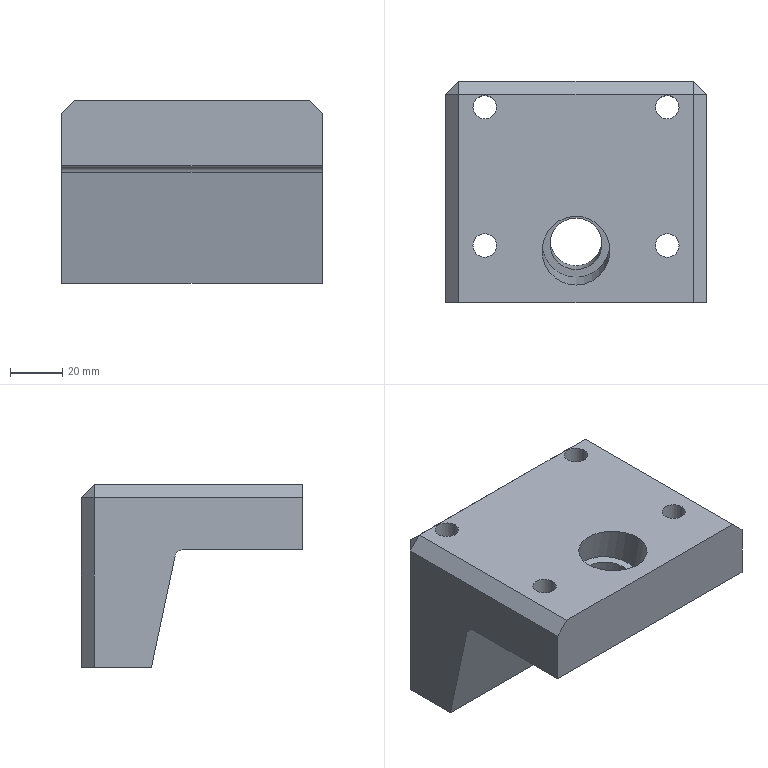Part | STEP file | P011002S001-009 | 1 solid | 31 faces | box 100 x 85 x 70 mm | volume 323771 mm3 | plane 20 | cylinder 11 | commonest cylinder face diameters 9 x4 14 x4 6 x1 20 x1 26 x1